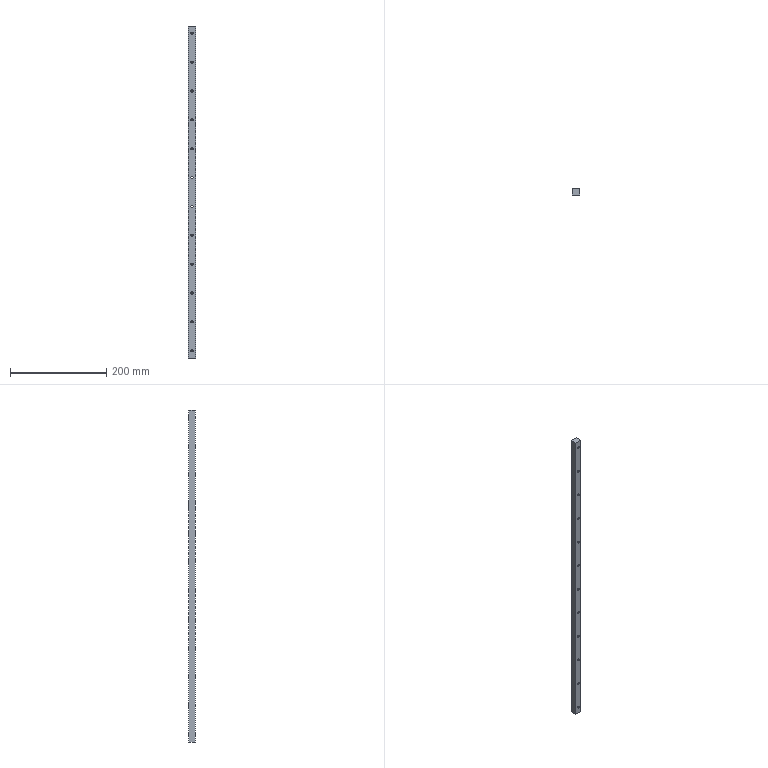Part | STEP file | PN_0081 15 guide rail, X crossbeam | 1 solid | 66 faces | box 15 x 14 x 690 mm | volume 140414 mm3 | cylinder 48 | plane 18 | commonest cylinder face diameters 4.5 x24 8 x24